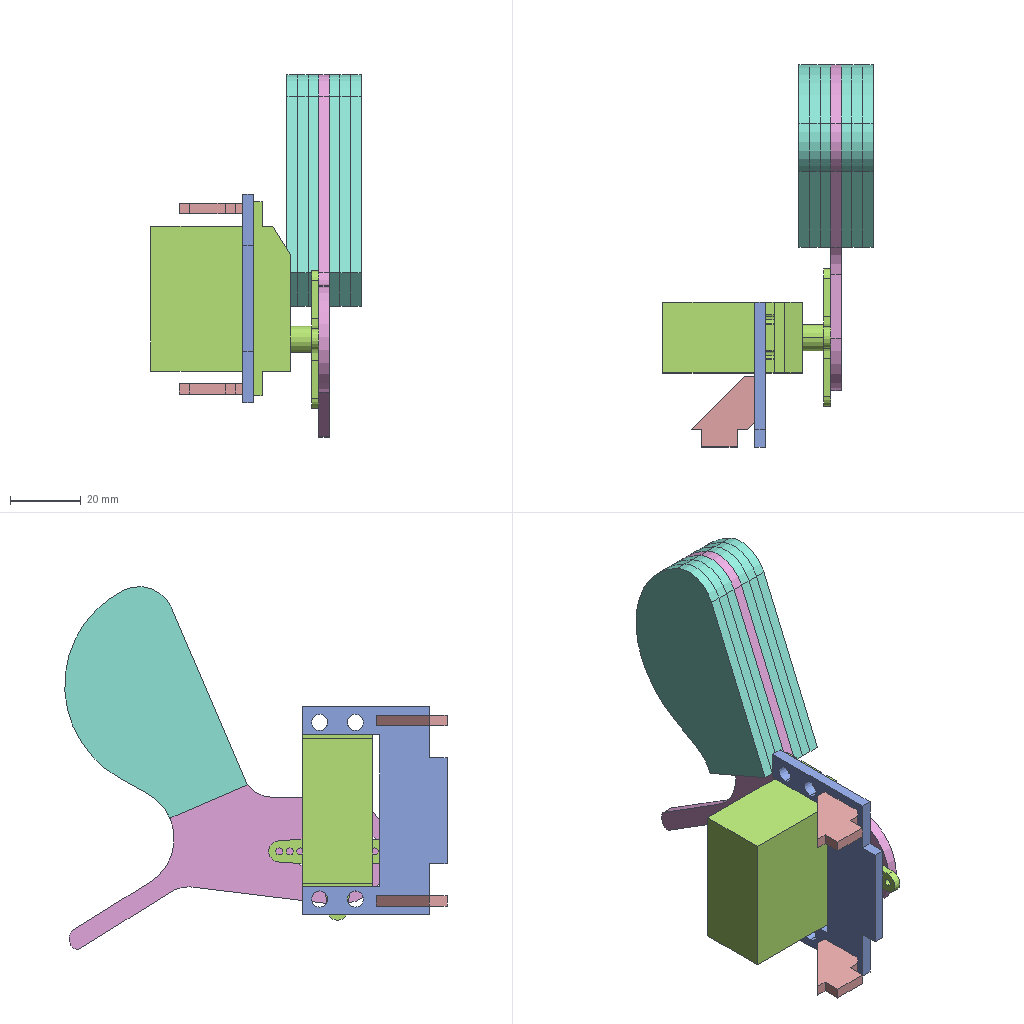Assembly | SolidWorks | 5 different items | 11 placed | box 60 x 108 x 103 mm
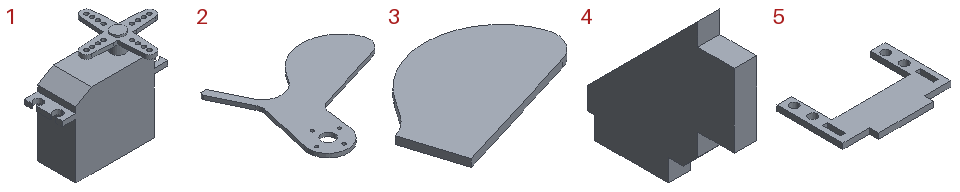Parts list (item | quantity | size | volume | features):
1 | x1 | 58.5 x 39 x 48.5 mm | 33649 mm3 | features ICE 6, Fillet 2, Chamfer 1, Extrusion 1, MirrorPattern 1
2 | x1 | 100.288 x 93 x 3 mm | 11352 mm3 | features ICE 4, Fillet 2, BaseBody 1, HoleWzd 1
3 | x6 | 66.131 x 48.568 x 3 mm | 6184 mm3 | features ICE 4, Fillet 2, BaseBody 1
4 | x2 | 3 x 20 x 21 mm | 706.5 mm3 | features Chamfer 2, ICE 2, Extrusion 1
5 | x1 | 59 x 41 x 3 mm | 3617 mm3 | features ICE 2, Extrusion 1
Mates (type | each side: item.copy, entity, surface, feature):
Coincident | 1.1 edge | 5.1 face cylinder Boss-Extrude1
Concentric | 1.1 face cylinder Cut-Extrude1 | 5.1 face cylinder Boss-Extrude1
Coincident | 1.1 face plane Boss-Extrude2 | 5.1 face plane Boss-Extrude1
Concentric | 2.1 face cylinder Imported1 | 1.1 face cylinder Boss-Extrude3
Coincident | 2.1 face plane Imported1 | 1.1 face plane Boss-Extrude3
Coincident | 2.1 face plane Imported1 | 3.1 face plane Imported1
Concentric | 2.1 face cylinder Imported1 | 3.1 face cylinder Imported1 | 2 times
Coincident | 2.1 face plane Imported1 | 3.2 face plane Imported1
Concentric | 2.1 face cylinder Imported1 | 3.2 face cylinder Imported1 | 2 times
DistanceDim | assembly plane | 5.1 face plane Boss-Extrude1
Coincident | 5.1 face plane Boss-Extrude1 | assembly plane | 2 times
Width | 4.1 face plane Boss-Extrude1 | 4.1 face plane Boss-Extrude1 | 5.1 face plane Cut-Extrude1 | 5.1 face plane Cut-Extrude1
Coincident | 4.1 face plane Boss-Extrude1 | 5.1 face plane Boss-Extrude1
Coincident | 4.1 face plane Boss-Extrude2 | 5.1 face plane Cut-Extrude1
Width | 4.2 face plane Boss-Extrude1 | 4.2 face plane Boss-Extrude1 | 5.1 face plane Cut-Extrude1 | 5.1 face plane Cut-Extrude1
Coincident | 5.1 face plane Boss-Extrude1 | 4.2 face plane Boss-Extrude1 | 2 times